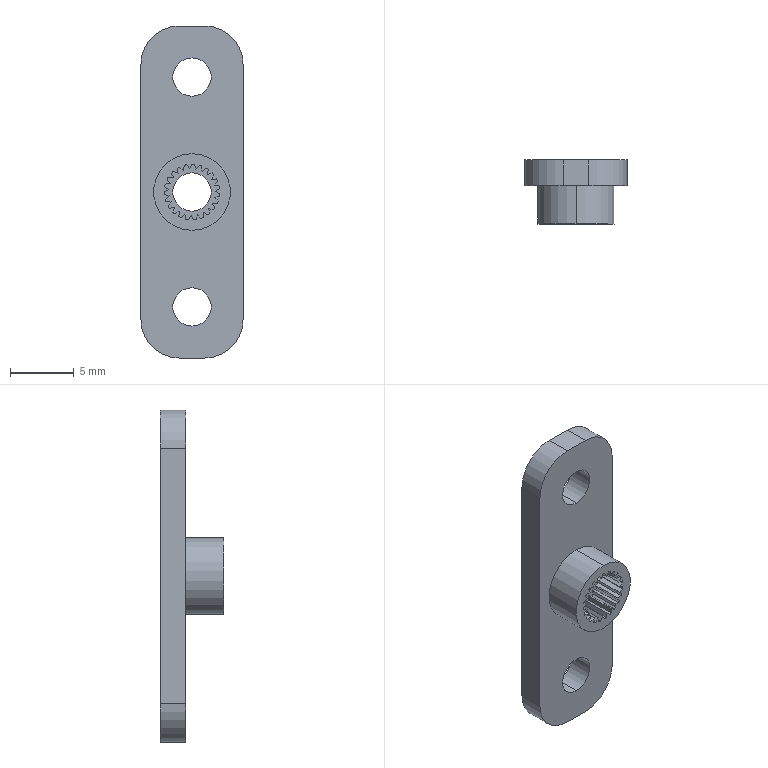Part | SolidWorks | features ICE 2, CombineBodies 1, Extrusion 1, MoveCopyBody 1, Stock 1 | 1 solid | 89 faces | box 8 x 5 x 26 mm | volume 406.224 mm3 | plane 54 | cylinder 35 | commonest cylinder face diameters 4.361 x23 3 x6 6 x6